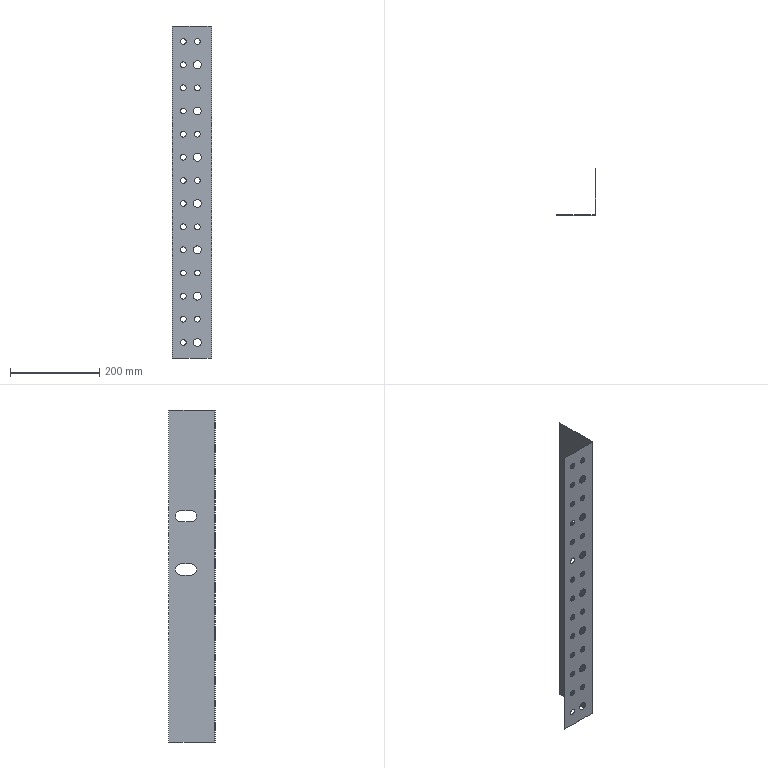Part | STEP file | 64524313 | 1 solid | 82 faces | box 89 x 104.75 x 746 mm | volume 102676 mm3 | cylinder 62 | plane 20 | commonest cylinder face diameters 13 x42 18 x14 25 x4 1.6 x1 3.1 x1